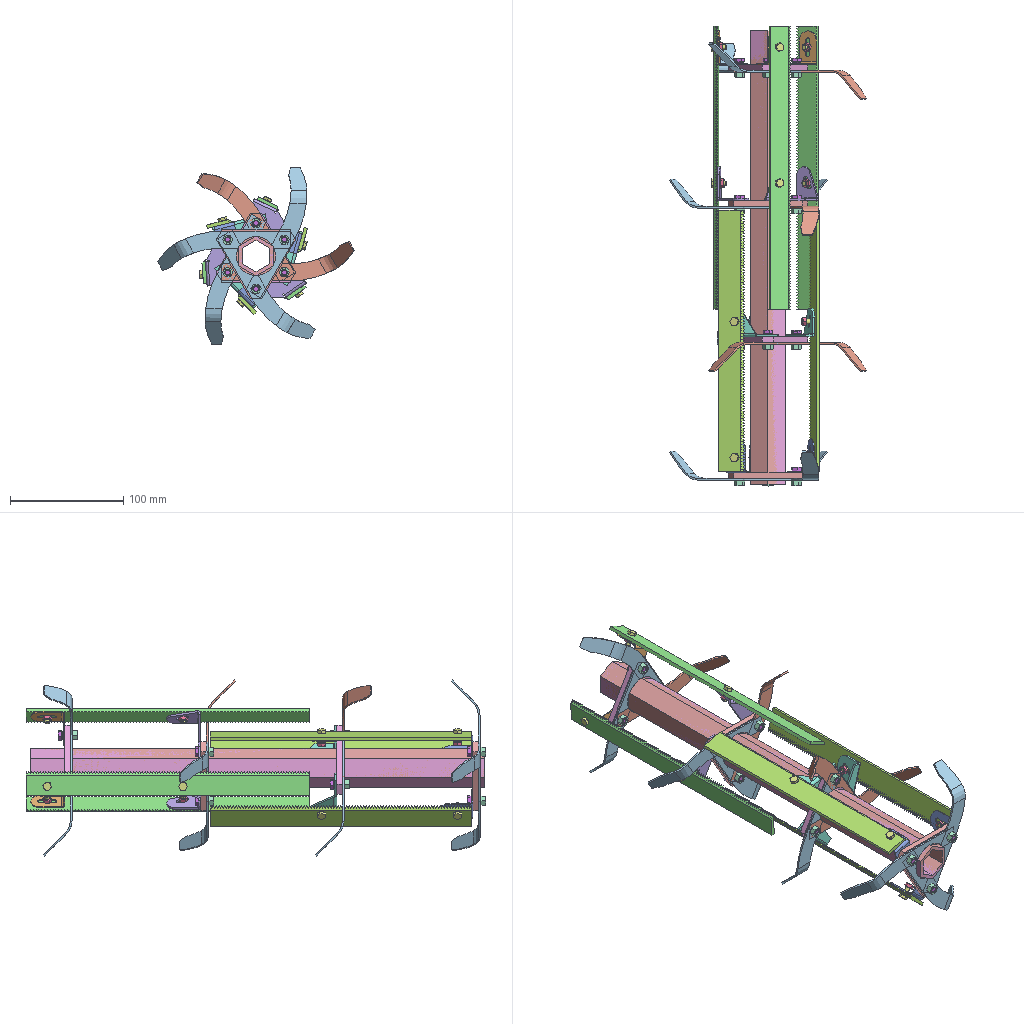Assembly | SolidWorks | 13 different items | 81 placed | box 174 x 406 x 156 mm
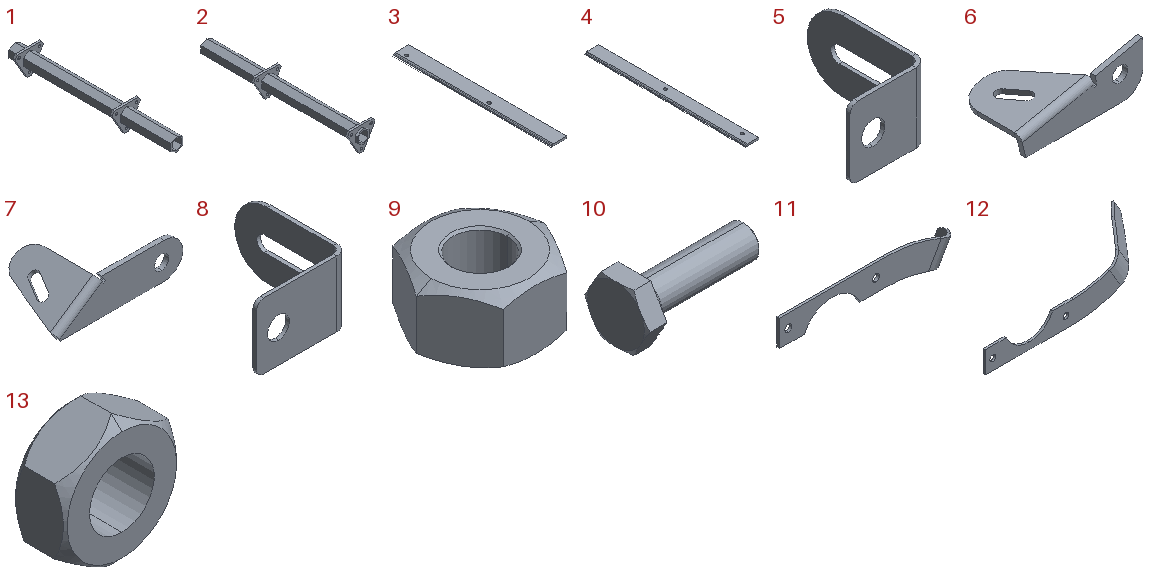Parts list (item | quantity | size | volume | features):
1 | x1 | 70 x 400 x 60.622 mm | 130008 mm3 | features ICE 5, Extrusion 1, LPattern 1
2 | x1 | 70 x 400 x 60.622 mm | 130008 mm3 | features ICE 5, Extrusion 1, LPattern 1
3 | x3 | 23 x 230.294 x 3 mm | 14437 mm3 | features Cut 2, Chamfer 1, Extrusion 1, ICE 1, LPattern 1
4 | x3 | 21 x 250 x 3 mm | 14340 mm3 | features ICE 2, Chamfer 1, Cut 1, Extrusion 1, LPattern 1, MirrorPattern 1
5 | x3 | 20 x 30 x 18 mm | 730.964 mm3 | features Fillet 2, ICE 2, EdgeFlange 1, FlatPattern 1, SMBaseFlange 1, SheetMetal 1
6 | x3 | 48.042 x 25.072 x 17.984 mm | 2002 mm3 | features Fillet 3, ICE 3, Cut 1, EdgeFlange 1, FlatPattern 1, SMBaseFlange 1, SheetMetal 1
7 | x3 | 53.504 x 30 x 15 mm | 2061 mm3 | features ICE 3, Cut 2, Fillet 2, EdgeFlange 1, FlatPattern 1, SMBaseFlange 1, SheetMetal 1
8 | x3 | 25 x 30 x 18 mm | 820.964 mm3 | features Fillet 2, ICE 2, EdgeFlange 1, FlatPattern 1, SMBaseFlange 1, SheetMetal 1
9 | x12 | 11.547 x 10 x 5.7 mm | 373.519 mm3 | features RevCut 4, Chamfer 2, Boss 1, Extrusion 1, LPattern 1
10 | x25 | 12.125 x 6.143 x 5.32 mm | 120.535 mm3 | features RevCut 3, Boss 1, Chamfer 1, Extrusion 1, Fillet 1, LPattern 1
11 | x4 | 116.818 x 25.618 x 34.656 mm | 2408 mm3 | features Chamfer 2, FlatPattern 2, Cut 1, ICE 1, MirrorSolid 1, SM3dBend 1, SMBaseFlange 1, SheetMetal 1
12 | x8 | 116.818 x 25.618 x 34.656 mm | 2408 mm3 | features Chamfer 2, Cut 1, FlatPattern 1, ICE 1, SM3dBend 1, SMBaseFlange 1, SheetMetal 1
13 | x12 | 7 x 3.2 x 8.083 mm | 93.048 mm3 | features Extrusion 1, ICE 1, RevCut 1
Mates (type | each side: item.copy, entity, surface, feature):
Coincident | 2.1 plane | assembly plane | 3 times
Coincident | 2.1 face plane Boss-Extrude1 | 1.1 face plane Boss-Extrude1
Coincident | 2.1 edge | 1.1 edge
Coincident | 2.1 face plane LPattern1 | 5.1 face plane Base-Flange1
Coincident | 1.1 face plane LPattern1 | 6.1 face plane Base-Flange1
Concentric | 1.1 face cylinder Cut-Extrude2 | 6.1 face cylinder Cut-Extrude6
Concentric | 2.1 face cylinder Cut-Extrude2 | 7.1 face cylinder Cut-Extrude6
Concentric | 1.1 face cylinder Cut-Extrude2 | 8.1 face cylinder Cut-Extrude4
Parallel | 2.1 face plane LPattern1 | 1.1 face plane LPattern1
Concentric | 2.1 face cylinder Cut-Extrude2 | 5.1 face cylinder Cut-Extrude4
Concentric | 3.1 face cylinder Cut-Extrude1 | 13.1 face cylinder Cut-Extrude1
Concentric | 2.1 face cylinder Cut-Extrude2 | 12.1 face cylinder Cut-Extrude1 | 2 times
Coincident | 2.1 face plane LPattern1 | 12.1 face plane Base-Flange1
Coincident | 8.1 face plane Edge-Flange1 | 13.2 face plane Boss-Extrude1
Concentric | 3.1 face cylinder Cut-Extrude1 | 10.1 face cylinder BaseBody
Coincident | 3.1 face plane Boss-Extrude1 | 10.1 face plane BaseHead
Concentric | 5.1 edge | 10.2 face cylinder BaseBody
Coincident | 5.1 face plane Base-Flange1 | 10.2 face plane BaseHead
Concentric | 10.2 face cylinder BaseBody | 9.1 face cylinder BaseNut
Coincident | 12.2 face plane Base-Flange1 | 9.1 face plane BaseNut
Coincident | 6.1 face plane Base-Flange1 | 10.3 face plane BaseHead
Concentric | 3.1 face cylinder Cut-Extrude1 | 10.4 face cylinder BaseBody
Coincident | 3.1 face plane Boss-Extrude1 | 10.4 face plane BaseHead
Concentric | 1.1 face cylinder Cut-Extrude2 | 10.3 face cylinder BaseBody
Coincident | 4.1 face plane Boss-Extrude1 | 10.5 face plane BaseHead
Concentric | 6.2 face cylinder Cut-Extrude6 | 10.6 face cylinder BaseBody
Coincident | 6.2 face plane Base-Flange1 | 10.6 face plane BaseHead
Concentric | 10.6 face cylinder BaseBody | 9.2 face cylinder BaseNut
Concentric | 13.2 face cylinder Cut-Extrude1 | 10.7 face cylinder BaseBody
Concentric | 10.6 face cylinder BaseBody | 12.3 edge
Concentric | 10.8 face cylinder BaseBody | 12.3 face cylinder Cut-Extrude1
Coincident | 1.1 face plane LPattern1 | 12.3 face plane Base-Flange1
Coincident | 2.1 face plane LPattern1 | 12.4 face plane Base-Flange1
Concentric | 10.9 face cylinder BaseBody | 12.5 edge
Concentric | 10.10 face cylinder BaseBody | 12.5 face cylinder Cut-Extrude1
Coincident | 2.1 face plane LPattern1 | 12.5 face plane Base-Flange1
Concentric | 10.11 face cylinder BaseBody | 12.6 edge
Concentric | 10.12 face cylinder BaseBody | 12.6 edge
Coincident | 1.1 face plane Boss-Extrude2 | 12.6 face plane Base-Flange1
Coincident | 8.1 face plane Edge-Flange1 | 4.1 face plane Boss-Extrude1
Coincident | 4.1 face plane Boss-Extrude1 | 10.7 face plane BaseHead
Parallel | 2.1 face plane LPattern1 | 7.1 face plane Base-Flange1
Coincident | 13.3 face plane Boss-Extrude1 | 7.2 face plane Edge-Flange1
Coincident | 2.1 face plane LPattern1 | 7.1 face plane Base-Flange1
Coincident | 1.1 face plane Boss-Extrude2 | 8.1 face plane Base-Flange1
Concentric | 10.13 face cylinder BaseBody | 11.1 edge
Concentric | 10.8 face cylinder BaseBody | 11.1 edge
Coincident | 1.1 face plane LPattern1 | 11.1 face plane Mirror1
Concentric | 10.13 face cylinder BaseBody | 11.2 edge
Concentric | 10.6 face cylinder BaseBody | 11.2 face cylinder Mirror1
Coincident | 1.1 face plane LPattern1 | 11.2 face plane Mirror1
Coincident | 2.1 face plane LPattern1 | 11.3 face plane Mirror1
Concentric | 10.9 edge | 11.3 edge
Concentric | 10.14 face cylinder BaseBody | 11.3 edge
Concentric | 10.10 face cylinder BaseBody | 12.4 edge
Concentric | 10.14 face cylinder BaseBody | 12.4 face cylinder Cut-Extrude1
Concentric | 10.15 face cylinder BaseBody | 11.4 edge
Concentric | 10.12 face cylinder BaseBody | 11.4 face cylinder Mirror1
Coincident | 1.1 face plane Boss-Extrude2 | 11.4 face plane Mirror1
Concentric | 13.4 face cylinder Cut-Extrude1 | 10.4 face cylinder BaseBody
Concentric | 10.15 face cylinder BaseBody | 12.7 face cylinder Cut-Extrude1
Concentric | 10.11 edge | 12.7 face cylinder Cut-Extrude1
Coincident | 1.1 face plane Boss-Extrude2 | 12.7 face plane Base-Flange1
Coincident | 5.1 face plane Edge-Flange1 | 3.1 face plane Boss-Extrude1
Slot | 10.1 face cylinder BaseBody | 5.1 face plane Cut-Extrude5
Parallel | 3.1 face plane Cut-Extrude3 | 1.1 face plane LPattern1
PlanarAngleDim | 3.1 face plane Boss-Extrude1 | 2.1 face plane LPattern1
Parallel | 8.1 face plane Edge-Flange1 | 4.1 face plane Boss-Extrude2
Parallel | 7.1 face plane Edge-Flange1 | 4.1 face plane Boss-Extrude1